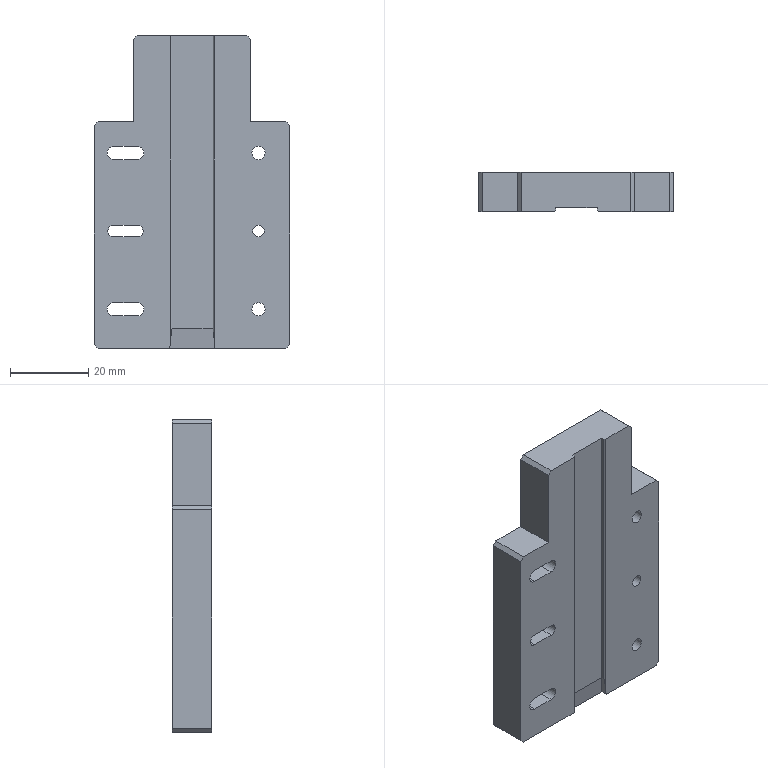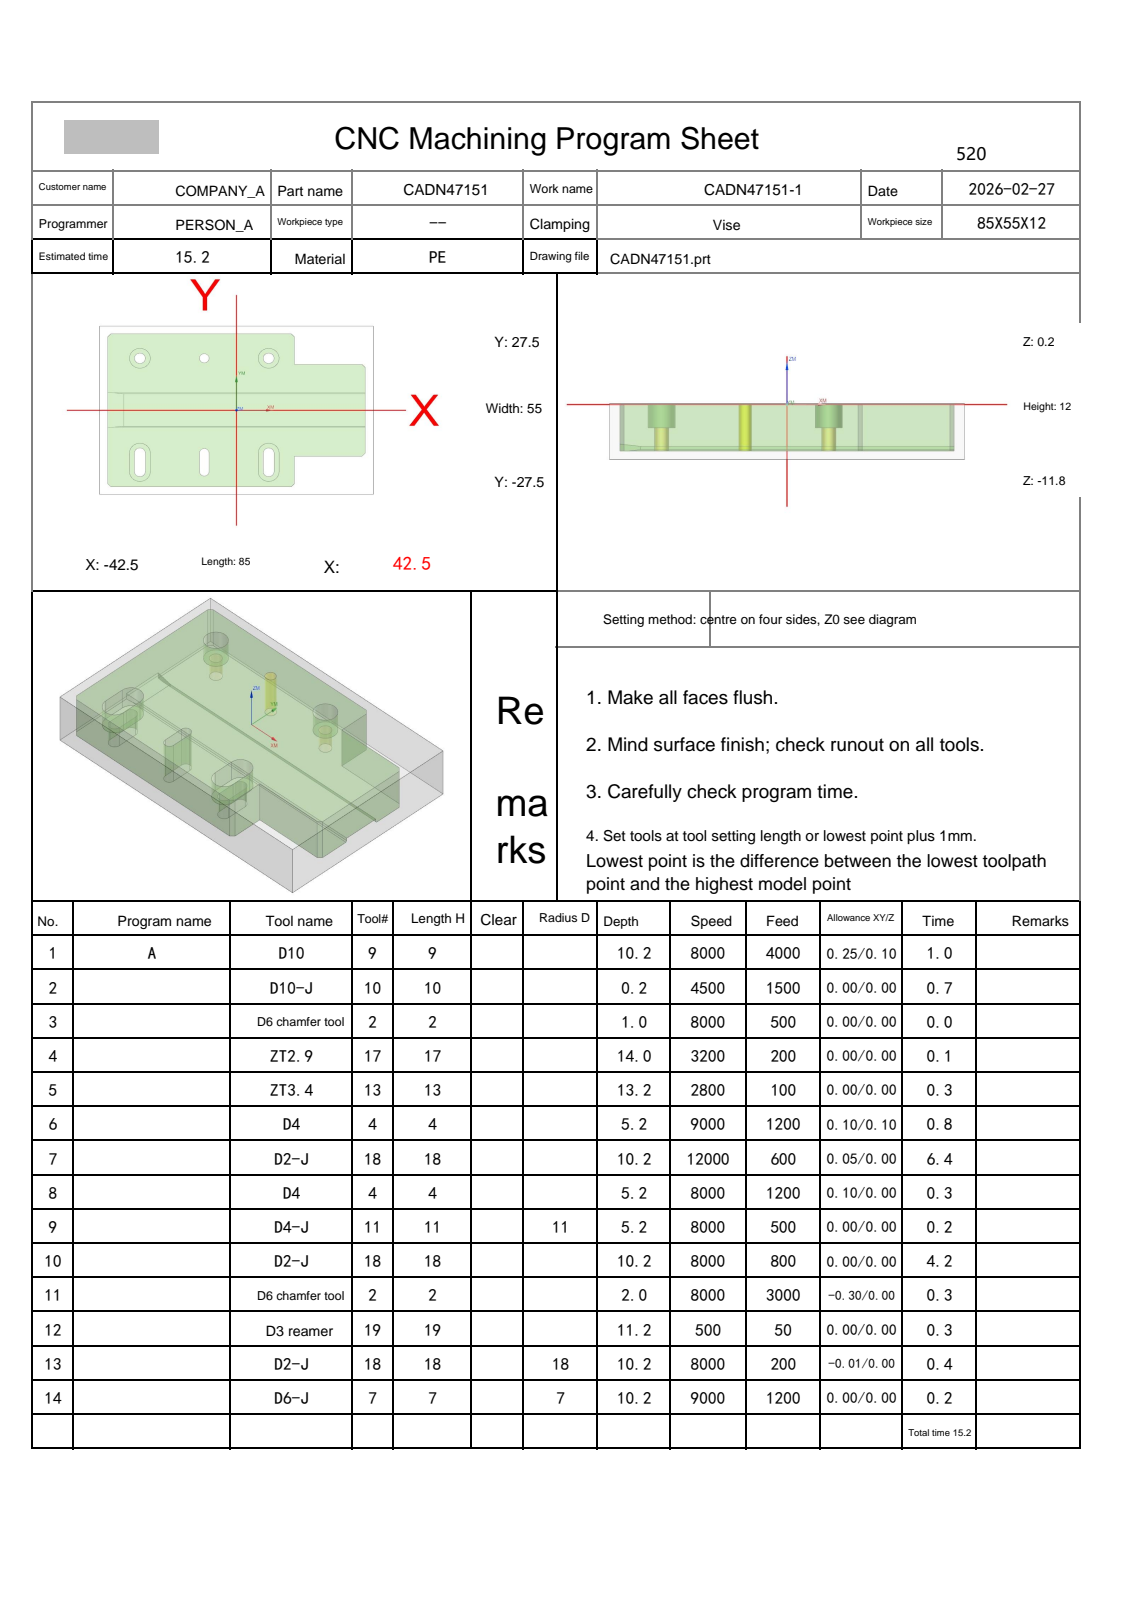NC program | NX | posted by the shop | part box 50 x 10 x 80 mm
Lines 1 to 1266 of 8100:
%
O0001
(Machine time: 17.84 MIN)
(===Total Tool:10===)
(T9=D10     D=10.  R=0.   D-  H09 Z=-10.  )
(T10=D10-J  D=10.  R=0.   D-  H10 Z=0.    )
(T2=D6 chamfer tool   D=6.   R=0.   D-  H02 Z=-1.8  )
(T17=ZT2.9  D=2.9  DR_a=120 D-  H17 Z=-13.84)
(T13=ZT3.4  D=3.4  DR_a=118 D-  H13 Z=-13.02)
(T4=D4      D=4.   R=0.   D-  H04 Z=-5.   )
(T18=D2-J   D=2.   R=0.   D-  H18 Z=-10.  )
(T11=D4-J   D=4.   R=0.   D11 H11 Z=-5.   )
(T19=D3 reamer   D=3.   DR_a=180 D-  H19 Z=-11.  )
(T7=D6-J    D=6.   R=0.   D7  H07 Z=-10.  )
G80 G90 G17 G49 G40
G91 G28 Z0
M01
N1 T09 M06
(D10  D=10. R=0. H=09 ce=0.25 di=0.10)
G00 G90 G54 X53.977 Y1.05 M03 S8000
G43 H09 Z50.
M08
Z-8.
G01 X53.878 Y1.032 Z-8.625 F4000.
X53.78 Y1.014 Z-8.872
X53.682 Y.996 Z-9.054
X53.583 Y.978 Z-9.2
X53.485 Y.96 Z-9.323
X53.387 Y.942 Z-9.428
X53.288 Y.924 Z-9.52
X53.19 Y.906 Z-9.6
X53.092 Y.888 Z-9.67
X52.993 Y.87 Z-9.732
X52.895 Y.852 Z-9.786
X52.796 Y.834 Z-9.833
X52.698 Y.816 Z-9.874
X52.6 Y.797 Z-9.908
X52.501 Y.779 Z-9.936
X52.403 Y.761 Z-9.96
X52.305 Y.743 Z-9.977
X52.206 Y.725 Z-9.99
X52.108 Y.707 Z-9.997
X52.01 Y.689 Z-10.
X49.894 Y.301
G03 X49.531 Y.025 I.097 J-.504
X49.097 Y-3.1 I11.047 J-3.125
G01 Y-3.168
G03 X48.997 Y-11.593 I354.863 J-8.424
X49. Y-13.006 I354.963 J0.0
G02 X49.015 Y-17.868 I-787.443 J-4.861
X48.97 Y-26.356 I-787.458 J0.0
X43.827 Y-33.039 I-7.224 J.238
X38.212 Y-33.904 I-5.806 J19.054
X29.259 Y-34.006 I-8.953 J392.015
X27.063 Y-34. I0.0 J392.117
G01 X-41.069 Y-33.984
X-41.096
G02 X-48.042 Y-28.819 I0.0 J7.254
X-48.914 Y-22.955 I19.689 J5.924
X-49.003 Y-13.772 I474.862 J9.182
X-49. Y-12.005 I474.951 J0.0
G01 X-48.984 Y26.069
Y26.096
G02 X-43.819 Y33.042 I7.254 J0.0
X-37.955 Y33.914 I5.924 J-19.689
X-28.772 Y34.003 I9.182 J-474.862
X-27.005 Y34. I0.0 J-474.951
G01 X41.069 Y33.984
X41.096
G02 X48.042 Y28.819 I0.0 J-7.254
X48.914 Y22.954 I-19.689 J-5.924
X49.021 Y10.694 I-707.018 J-12.261
X48.963 Y1.656 I-707.124 J0.0
G03 X48.498 Y-9.252 I127.706 J-10.908
X48.505 Y-10.615 I128.171 J0.0
G02 X48.521 Y-15.637 I-779.152 J-5.022
X48.465 Y-25.004 I-779.168 J0.0
X43.679 Y-31.936 I-7.896 J.334
X37.464 Y-33.313 I-6.835 J16.126
X28.561 Y-33.517 I-8.903 J194.629
X25.918 Y-33.499 I0.0 J194.833
G01 X-39.655 Y-33.482
G02 X-47.019 Y-28.497 I.029 J7.975
X-48.313 Y-22.465 I16.584 J6.714
X-48.52 Y-13.11 I211.138 J9.355
X-48.499 Y-10.118 I211.345 J0.0
G01 X-48.48 Y24.705
G02 X-43.679 Y31.935 I7.926 J-.053
X-37.465 Y33.313 I6.835 J-16.119
X-28.138 Y33.52 I9.327 J-210.133
X-25.168 Y33.499 I0.0 J-210.34
G01 X39.655 Y33.482
G02 X47.019 Y28.497 I-.029 J-7.975
X48.313 Y22.465 I-16.584 J-6.714
X48.52 Y13.11 I-211.138 J-9.355
X48.499 Y10.118 I-211.346 J0.0
X48.522 Y7.551 I-146.57 J-2.567
X48.169 Y-2.608 I-146.592 J0.0
G03 X48. Y-12.795 I306.009 J-10.187
G01 X48.001 Y-13.507
G02 X48.018 Y-17.014 I-360.035 J-3.507
X47.953 Y-23.855 I-360.052 J0.0
X42.658 Y-31.323 I-8.682 J.544
X36.005 Y-32.794 I-7.383 J17.622
X27.174 Y-33.012 I-8.83 J178.054
X24.909 Y-32.998 I0.0 J178.273
G01 X-38.241 Y-32.983
X-38.277
G02 X-46.322 Y-27.659 I0.0 J8.741
X-47.793 Y-21.005 I17.608 J7.383
X-48.014 Y-12.022 I182.708 J8.983
X-47.998 Y-9.609 I182.929 J0.0
G01 X-47.973 Y23.49
G02 X-42.659 Y31.322 I8.718 J-.196
X-36.005 Y32.793 I7.383 J-17.609
X-27.02 Y33.014 I8.985 J-182.767
X-24.609 Y32.998 I0.0 J-182.988
G01 X38.29 Y32.982
G02 X46.322 Y27.659 I-.01 J-8.737
X47.793 Y21.005 I-17.609 J-7.383
X48.014 Y12.022 I-182.711 J-8.983
X47.998 Y9.609 I-182.931 J0.0
X48.001 Y8.479 I-198.39 J-1.13
X47.65 Y-3.318 I-198.393 J0.0
G03 X47.478 Y-18.337 I654.031 J-15.019
X47.487 Y-21.806 I654.204 J0.0
G02 X47.49 Y-22.034 I-9.468 J-.228
X41.526 Y-30.832 I-9.471 J0.0
X34.809 Y-32.273 I-7.637 J19.219
X25.573 Y-32.513 I-9.236 J177.333
X23.214 Y-32.497 I0.0 J177.573
G01 X-37.036 Y-32.479
X-37.056
G02 X-45.825 Y-26.538 I0.0 J9.443
X-47.29 Y-19.574 I19.56 J7.75
X-47.517 Y-9.838 I208.749 J9.736
X-47.498 Y-7.028 I208.976 J0.0
G01 X-47.481 Y21.972
Y22.05
G02 X-41.538 Y30.826 I9.45 J0.0
X-34.574 Y32.29 I7.75 J-19.561
X-24.836 Y32.517 I9.738 J-208.817
X-22.028 Y32.498 I0.0 J-209.044
G01 X36.972 Y32.481
X37.05 Y32.482
G02 X45.826 Y26.538 I0.0 J-9.45
X47.29 Y19.574 I-19.562 J-7.75
X47.519 Y9.517 I-221.257 J-10.057
X47.178 Y-2.769 I-221.486 J0.0
G03 X46.979 Y-18.281 I604.501 J-15.512
X46.983 Y-20.656 I604.7 J0.0
G01 X46.985 Y-20.853
G02 X44.669 Y-27.375 I-10.342 J0.0
X38.251 Y-31.072 I-8.949 J8.117
X30.461 Y-31.919 I-7.882 J36.235
X20.214 Y-32. I-10.248 J651.166
X18.862 Y-31.998 I0.0 J651.247
G01 X-35.788 Y-31.978
X-35.917 Y-31.979
G02 X-43.02 Y-29.073 I0.0 J10.133
X-46.222 Y-22.617 I9.557 J8.763
X-46.941 Y-14.714 I43.079 J7.902
G01 Y-14.611
G02 X-47.002 Y-5.696 I655.87 J8.915
X-46.998 Y-3.611 I655.93 J0.0
G01 X-46.976 Y20.839
Y20.944
G02 X-43.67 Y28.392 I10.042 J0.0
X-37.126 Y31.321 I8.642 J-10.533
X-28.922 Y31.966 I8.204 J-51.84
X-28.361 Y31.963 I0.0 J-52.485
G01 X-18.611 Y31.998
X35.839 Y31.976
X35.943 Y31.977
G02 X43.156 Y28.924 I0.0 J-10.049
X46.242 Y22.511 I-9.842 J-8.686
X46.943 Y14.63 I-43.943 J-7.881
G01 Y14.503
G02 X46.985 Y9.735 I-270.462 J-4.768
X46.652 Y-3.693 I-270.504 J0.0
G03 X46.469 Y-19.857 I958.738 J-18.923
G01 Y-19.878
G02 X43.937 Y-26.81 I-10.755 J0.0
X37.405 Y-30.524 I-9.213 J8.603
X29.071 Y-31.421 I-8.335 J38.26
X18.93 Y-31.5 I-10.14 J655.907
X17.471 Y-31.498 I0.0 J655.986
G01 X-34.529 Y-31.479
X-34.6
G02 X-40.239 Y-30.093 I0.0 J12.161
X-43.188 Y-28.258 I1.605 J5.867
X-45.308 Y-24.357 I4.303 J4.865
X-46.419 Y-14.388 I46.553 J10.234
X-46.5 Y-4.081 I657.762 J10.307
X-46.498 Y-2.488 I657.843 J0.0
G01 X-46.471 Y19.761
G02 X-45.092 Y25.246 I11.999 J-.101
X-43.711 Y27.713 I5.537 J-1.479
G01 X-42.085 Y29.248
G02 X-39.342 Y30.31 I3.668 J-5.402
X-29.122 Y31.426 I10.327 J-47.201
X-19.247 Y31.5 I9.875 J-657.174
X-17.523 Y31.498 I0.0 J-657.249
G01 X34.527 Y31.479
X34.716 Y31.481
G02 X40.917 Y29.635 I0.0 J-11.339
X45.313 Y23.168 I-6.959 J-9.458
X46.376 Y15.411 I-30.851 J-8.178
X46.467 Y8.759 I-241.853 J-6.651
X46.172 Y-3.194 I-241.945 J0.0
G03 X45.97 Y-18.711 I841.279 J-18.691
G01 Y-18.771
G02 X43.979 Y-25.318 I-11.761 J0.0
X37.436 Y-29.748 I-9.705 J7.286
X29.635 Y-30.858 I-8.374 J30.89
X18.907 Y-31.009 I-10.728 J382.487
X15.987 Y-30.998 I0.0 J382.637
G01 X-33.363 Y-30.979
G02 X-38.013 Y-30.25 I.115 J15.922
X-38.514 Y-30.264 I-.502 J8.744
X-40.242 Y-30.092 I0.0 J8.758
G03 X-38.262 Y-30.272 I1.98 J10.806
X-37.667 Y-30.256 I0.0 J10.986
X-29.407 Y-30.607 I8.261 J97.074
X-27.82 Y-30.594 I0.0 J97.425
G01 X23.634 Y-30.58
G03 X24.704 Y-30.588 I1.071 J78.351
X33.664 Y-30.074 I0.0 J78.359
X40.558 Y-27.693 I-1.817 J16.438
X45.22 Y-20.113 I-6.075 J8.961
X45.6 Y-14.16 I-46.482 J5.954
X45.597 Y-13.63 I-46.861 J0.0
G02 X46.044 Y5.056 I741.844 J-8.393
G03 X46.1 Y8.875 I-130.374 J3.819
X45.784 Y17.948 I-130.43 J0.0
X44.034 Y24.942 I-19.775 J-1.23
X35.837 Y30.742 I-9.415 J-4.614
X29.577 Y31.103 I-6.261 J-54.029
X28.402 Y31.09 I0.0 J-54.39
G01 X-26.248 Y31.07
G03 X-26.865 Y31.073 I-.617 J-71.011
X-36.22 Y30.454 I0.0 J-71.014
G02 X-38.426 Y30.226 I-2.205 J10.558
X-39.125 Y30.248 I0.0 J10.786
G01 X-40.348 Y30.076
G02 X-38.165 Y30.269 I2.182 J-12.221
X-37.444 Y30.248 I0.0 J-12.415
G03 X-29.913 Y30.477 I-.343 J135.653
G02 X-17.911 Y30.602 I12.002 J-573.446
X-15.514 Y30.597 I0.0 J-573.572
G01 X29.736 Y30.574
G02 X30.362 Y30.58 I.626 J-30.941
X36.151 Y30.034 I0.0 J-30.947
X43.939 Y23.116 I-2.436 J-10.586
X45.373 Y15.731 I-23.454 J-8.387
X45.569 Y7.889 I-157.392 J-7.841
X45.42 Y1.036 I-157.587 J0.0
G03 X45.226 Y-10.074 I318.081 J-11.11
X45.25 Y-14.002 I318.275 J0.0
G02 X44.671 Y-19.744 I-58.173 J2.965
X37.39 Y-28.391 I-11.087 J1.946
X29.712 Y-29.87 I-8.649 J24.235
X20.007 Y-30.105 I-9.705 J200.151
X18.166 Y-30.097 I0.0 J200.386
G01 X17.2 Y-30.246
X-37.85 Y-30.25
G03 X-38.35 Y-30.75 I0.0 J-.5
X-38.119 Y-31.171 I.5 J0.0
G01 X-37.372 Y-31.648
X-35.701 Y-32.714 Z-9.9
X-35.361 Y-32.931
X-35.298 Y-32.965
X-35.232 Y-32.99
X-35.162 Y-33.005
X-35.091 Y-33.01
X15.407 Y-32.856
X15.491 Y-32.849
X15.573 Y-32.827
X15.649 Y-32.793
X15.719 Y-32.745
X17.018 Y-31.248 Z-10.
X17.913 Y-30.215
G02 X19.428 Y-29.888 I1.63 J-3.884
X27.197 Y-29.583 I9.717 J-148.644
G03 X35.168 Y-28.581 I-.47 J35.935
X41.784 Y-24.496 I-2.893 J12.085
X44.376 Y-17.974 I-10.749 J8.048
G01 X44.577 Y-16.551
X45.071 Y-15.359
X45.25 Y-14.002
X45.071 Y-15.359
G03 X43.532 Y-19.678 I31.519 J-13.668
G02 X35.394 Y-27.742 I-11.687 J3.654
X27.37 Y-29.028 I-8.8 J29.24
G03 X20.119 Y-29.381 I4.644 J-170.313
X19.579 Y-29.573 I.054 J-1.006
G01 X18.433 Y-30.056
X20.126 Y-29.304
G02 X24.435 Y-28.786 I4.653 J-20.498
G03 X32.477 Y-28.004 I-1.448 J56.619
X39.37 Y-24.881 I-2.445 J14.566
X43.163 Y-19.067 I-9.393 J10.273
G01 X43.711 Y-17.713
X44.547 Y-16.625
G03 X42.144 Y-20.306 I14.839 J-12.309
G02 X33.291 Y-27.106 I-12.178 J6.691
X25.48 Y-28.203 I-9.377 J38.403
G03 X20.68 Y-28.794 I.698 J-25.485
G01 X19.759 Y-29.454
X20.718 Y-28.749
G02 X24.207 Y-27.973 I4.129 J-10.327
G03 X31.46 Y-27.058 I-5.462 J72.542
X38.937 Y-23.434 I-2.695 J15.084
X42.344 Y-19.023 I-15.379 J15.399
X43.711 Y-17.713 I-23.663 J26.076
G02 X41.901 Y-19.405 I-20.641 J20.268
X38.549 Y-22.928 I-29.336 J24.562
X30.687 Y-26.561 I-10.91 J13.285
X23.882 Y-27.533 I-18.611 J106.014
G03 X21.213 Y-28.23 I.799 J-8.517
G01 X20.578 Y-28.832
G02 X23.057 Y-27.445 I3.203 J-2.816
X28.876 Y-26.461 I17.86 J-87.913
G03 X36.584 Y-23.687 I-2.784 J19.829
X40.888 Y-19.884 I-14.851 J21.148
G01 X41.625 Y-19.547
X42.339 Y-18.999
G02 X40.781 Y-19.912 I-3.047 J3.411
G03 X37.595 Y-22.289 I39.735 J-56.585
G02 X28.754 Y-25.882 I-12.372 J17.771
G03 X23.192 Y-26.983 I11.673 J-73.551
X21.843 Y-27.549 I.98 J-4.223
G01 X21.24 Y-28.204
G02 X22.181 Y-27.271 I4.795 J-3.9
X25.782 Y-26.085 I5.47 J-10.547
G03 X32.485 Y-24.402 I-8.054 J46.254
X38.795 Y-20.816 I-8.901 J23.008
G02 X39.868 Y-20.136 I4.281 J-5.568
G03 X40.959 Y-19.822 I-.116 J2.464
G02 X39.626 Y-20.19 I-1.762 J3.782
G03 X36.381 Y-21.916 I9.596 J-21.955
G02 X27.58 Y-25.153 I-14.713 J26.42
G03 X22.998 Y-26.476 I4.424 J-23.917
X22.425 Y-26.825 I1.547 J-3.186
G01 X21.861 Y-27.527
G02 X24.152 Y-25.798 I3.489 J-2.241
X29.571 Y-24.234 I23.148 J-70.025
G03 X37.374 Y-20.864 I-10.099 J34.105
G02 X38.733 Y-20.25 I5.626 J-10.641
G01 X39.841 Y-20.139
G03 X38.186 Y-20.331 I5.071 J-51.09
X34.274 Y-21.93 I9.978 J-29.979
G02 X26.523 Y-24.536 I-22.319 J53.569
G03 X22.908 Y-26.066 I2.815 J-11.686
X22.43 Y-26.814 I1.245 J-1.321
G02 X23.885 Y-25.296 I2.54 J-.977
X27.912 Y-23.757 I10.204 J-20.655
G03 X36.144 Y-20.679 I-22.277 J72.129
G01 X37.427 Y-20.25
X38.677
G03 X38.02 Y-20.225 I-.657 J-8.735
X34.671 Y-20.891 I0.0 J-8.759
G02 X26.073 Y-23.868 I-231.278 J654.106
G03 X23.063 Y-25.515 I2.739 J-8.58
G01 X22.709 Y-26.252
G02 X23.224 Y-25.284 I3.786 J-1.393
X26.174 Y-23.52 I5.738 J-6.248
X35.259 Y-20.327 I64.878 J-170.115
G01 X35.587 Y-20.25
X37.237
G03 X36.388 Y-20.226 I-.848 J-14.798
X34.245 Y-20.382 I0.0 J-14.822
X25.181 Y-23.51 I11.561 J-48.193
X23.15 Y-25.05 I2.185 J-4.993
G01 X22.979 Y-25.655
G02 X24.108 Y-23.948 I2.467 J-.406
X28.539 Y-21.763 I9.789 J-14.261
X33.345 Y-20.25 I16.134 J-42.871
G01 X35.245
G03 X34.262 Y-20.227 I-.983 J-21.383
X32.06 Y-20.341 I0.0 J-21.405
X24.604 Y-23.169 I3.922 J-21.582
X23.221 Y-24.55 I1.951 J-3.336
G01 X23.124 Y-25.111
G02 X24.099 Y-23.342 I2.393 J-.165
X28.677 Y-20.921 I8.832 J-11.163
X30.977 Y-20.25 I10.629 J-32.146
G01 X32.927
G03 X31.937 Y-20.229 I-.989 J-23.118
X29.846 Y-20.324 I0.0 J-23.139
X24. Y-23.025 I2.001 J-12.006
X23.247 Y-24.086 I1.565 J-1.909
G01 X23.211 Y-24.605
X23.21 Y-24.544
G02 X24.054 Y-22.765 I2.295 J0.0
X28.894 Y-20.25 I7.243 J-8.022
G01 X30.544
G03 X29.724 Y-20.226 I-.82 J-13.844
X27.88 Y-20.349 I0.0 J-13.869
X23.602 Y-22.885 I1.565 J-7.517
X23.231 Y-23.83 I1.019 J-.946
X23.248 Y-24.05 I1.39 J0.0
G02 X23.238 Y-23.849 I2.073 J.201
X23.892 Y-22.334 I2.083 J0.0
X27.365 Y-20.25 I5.343 J-4.968
G01 X28.615
G03 X28.002 Y-20.226 I-.613 J-7.851
X26.465 Y-20.377 I0.0 J-7.875
X23.277 Y-22.872 I1.292 J-4.936
G01 X23.25 Y-23.554
G02 X23.237 Y-23.318 I2.218 J.236
X24.008 Y-21.632 I2.231 J0.0
X26.271 Y-20.25 I3.751 J-3.599
G01 X27.171
G03 X26.722 Y-20.225 I-.448 J-4.025
X25.027 Y-20.597 I0.0 J-4.05
X23.256 Y-22.421 I1.517 J-3.245
G01 X23.25 Y-22.971
G02 X23.239 Y-22.76 I2.093 J.211
X24.038 Y-21.11 I2.104 J0.0
X25.5 Y-20.25 I2.516 J-2.605
G01 X26.2
G03 X25.841 Y-20.227 I-.36 J-2.784
X23.257 Y-21.936 I0.0 J-2.808
G01 X23.25 Y-22.436
X23.241 Y-22.252
G02 X24.101 Y-20.675 I1.876 J0.0
X25.212 Y-20.235 I1.111 J-1.181
X25.432 Y-20.25 I0.0 J-1.622
G03 X25.135 Y-20.228 I-.296 J-1.963
X23.25 Y-21.592 I0.0 J-1.985
G01 Y-21.942
X23.245 Y-21.812
G02 X24.186 Y-20.37 I1.576 J0.0
X24.722 Y-20.24 I.536 J-1.043
G01 X24.874 Y-20.25
G03 X24.655 Y-20.233 I-.22 J-1.447
X23.25 Y-21.285 I0.0 J-1.464
G01 Y-21.585
X23.241 Y-21.439
G02 X24.431 Y-20.249 I1.19 J0.0
G01 X24.482 Y-20.25
X24.322 Y-20.239
G03 X23.25 Y-21.052 I0.0 J-1.114
G01 Y-21.252
X23.245 Y-21.161
G02 X24.157 Y-20.249 I.911 J0.0
G01 X24.193 Y-20.25
X24.049 Y-20.237
G03 X23.249 Y-21.037 I0.0 J-.8
G01 X23.25 Y-21.072
X23.243 Y-20.972
G02 X23.966 Y-20.249 I.723 J0.0
G01 X24.003 Y-20.25
X23.887 Y-20.239
G03 X23.249 Y-20.877 I0.0 J-.637
G01 X23.25 Y-20.903
G03 X23.396 Y-21.257 I.52 J.008
G01 X24.326 Y-22.186
X25.727 Y-23.588 Z-9.9
X26.05 Y-23.911
X26.11 Y-23.962
X26.177 Y-24.003
X26.249 Y-24.033
X26.326 Y-24.051
X26.404 Y-24.057
X31.64
X32.487 Y-24.05
X33.335 Y-24.028
X34.181 Y-23.992
X35.028 Y-23.941
X35.873 Y-23.876
X36.716 Y-23.796
X37.559 Y-23.702
X38.399 Y-23.593
X39.238 Y-23.47
X40.074 Y-23.333
X40.908 Y-23.181
X44.284 Y-22.537
X44.472 Y-22.494
X44.657 Y-22.438
X44.837 Y-22.367
X45.011 Y-22.285
X45.179 Y-22.189
X45.339 Y-22.081
X45.491 Y-21.963
X45.634 Y-21.833
X45.767 Y-21.693
X45.89 Y-21.544
X46.001 Y-21.386
X46.1 Y-21.221
X46.293 Y-20.857
X46.474 Y-20.487
X46.642 Y-20.112
X46.798 Y-19.731
X46.94 Y-19.345
X47.07 Y-18.954
X47.637 Y-17.142
X47.785 Y-16.645
X47.919 Y-16.145
X48.039 Y-15.641
X48.146 Y-15.134
X48.239 Y-14.624
X48.317 Y-14.112
X48.382 Y-13.598
X48.432 Y-13.082
X48.468 Y-12.565
X48.49 Y-12.047
X48.498 Y-11.529
X48.491 Y-11.011
X48.404 Y-7.704
X48.395 Y-7.621
X48.372 Y-7.541
X48.336 Y-7.466
X48.288 Y-7.398
X48.23 Y-7.338
X47.741 Y-6.918
X46.237 Y-5.627 Z-10.
X45.364 Y-4.868
X45.25 Y-4.551
Y14.
G03 X44.295 Y20.269 I-64.76 J-6.658
X40.934 Y26.647 I-12.695 J-2.615
X34.403 Y29.733 I-8.117 J-8.723
X27.677 Y30.188 I-6.727 J-49.584
X26.874 Y30.181 I0.0 J-50.039
G01 X17.515 Y30.198
X17.203 Y30.246
X-35.297 Y30.248
G02 X-35.796 Y30.748 I0.0 J.5
X-35.565 Y31.17 I.5 J0.0
G01 X-34.815 Y31.649
X-33.143 Y32.714 Z-9.9
X-32.806 Y32.929
X-32.744 Y32.963
X-32.677 Y32.988
X-32.608 Y33.003
X-32.537 Y33.008
X14.756 Y32.957
X14.841 Y32.95
X14.924 Y32.928
X15.002 Y32.892
X15.073 Y32.843
X15.134 Y32.783
X15.172 Y32.74
X16.464 Y31.237 Z-10.
X17.262 Y30.316
G03 X18.433 Y30.056 I1.273 J2.967
X23.469 Y29.709 I5.036 J36.439
X24.116 Y29.715 I0.0 J36.785
G02 X24.988 Y29.719 I.872 J-90.757
X32.596 Y29.4 I0.0 J-90.761
X39.039 Y27.135 I-1.058 J-13.307
X43.449 Y20.606 I-7.497 J-9.817
X44.301 Y16.958 I-44.736 J-12.379
G01 X44.547 Y16.625
X45.071 Y15.359
G03 X44.199 Y17.14 I-6.362 J-2.011
G01 X42.792 Y21.117
G03 X33.867 Y28.601 I-11.099 J-4.172
X26.539 Y29.273 I-7.328 J-39.674
X26.209 Y29.271 I0.0 J-40.345
G02 X25.707 Y29.269 I-.501 J63.706
X19.594 Y29.563 I0.0 J63.708
G01 X18.433 Y30.056
G03 X22.768 Y28.962 I4.592 J9.063
G02 X30.418 Y28.544 I-14.028 J-326.874
X37.053 Y26.664 I-1.01 J-16.22
X42.159 Y20.737 I-6.518 J-10.777
G01 X43.287 Y18.137
G02 X44.322 Y16.918 I-5.747 J-5.925
G03 X43.115 Y18.344 I-11.421 J-8.444
G02 X41.219 Y21.633 I110.135 J65.669
G03 X32.496 Y27.674 I-11.08 J-6.68
X25.122 Y28.425 I-8.376 J-45.721
G02 X20.411 Y29.009 I.253 J21.335
G01 X19.592 Y29.564
G03 X21.039 Y28.688 I4.28 J5.434
X25.68 Y27.947 I5.396 J18.874
G02 X32.403 Y27.069 I-1.95 J-41.141
X40.702 Y21.123 I-3.122 J-13.12
G01 X41.896 Y19.339
G02 X43.279 Y18.145 I-4.841 J-7.01
G03 X41.69 Y19.516 I-8.895 J-8.71
G01 X39.097 Y22.491
G03 X30.773 Y26.866 I-10.796 J-10.433
X24.142 Y27.707 I-15.158 J-92.966
G02 X20.952 Y28.486 I.818 J10.275
G01 X20.336 Y29.041
G03 X23.141 Y27.557 I3.608 J3.425
X28.798 Y26.664 I16.159 J84.002
G02 X36.177 Y24.007 I-2.21 J-17.715
X40.124 Y20.435 I-14.101 J-19.547
G01 X40.648 Y19.951
G02 X41.823 Y19.394 I-1.267 J-4.192
G03 X40.556 Y19.991 I-2.702 J-4.097
G02 X37.971 Y22.063 I13.884 J19.968
G03 X28.869 Y26.158 I-11.992 J-14.495
G02 X23.188 Y27.207 I12.554 J83.849
X21.602 Y27.828 I1.926 J7.253
G01 X21.014 Y28.427
G03 X23.725 Y26.77 I3.808 J3.185
X29.313 Y25.529 I26.399 J105.711
G02 X37.554 Y21.601 I-4.26 J-19.544
G03 X39.599 Y20.171 I7.951 J9.195
G01 X39.616
G02 X40.636 Y19.956 I0.0 J-2.527
G03 X39.5 Y20.188 I-1.266 J-3.311
G02 X37.712 Y21.139 I3.535 J8.803
G03 X27.371 Y25.495 I-15.265 J-21.785
G02 X22.832 Y26.783 I4.215 J23.498
X21.665 Y27.762 I.904 J2.262
G03 X24.155 Y25.987 I3.788 J2.679
X29.442 Y24.455 I28.065 J86.957
G02 X36.833 Y21.056 I-8.878 J-29.045
G03 X38.461 Y20.25 I4.688 J7.415
G01 X38.485
G02 X39.596 Y20.171 I0.0 J-7.921
G03 X38.193 Y20.285 I-3.358 J-32.74
G02 X34.835 Y21.781 I6.016 J18.018
G03 X26.773 Y24.76 I-18.297 J-37.119
G02 X22.817 Y26.34 I3.388 J14.223
X22.425 Y26.825 I.539 J.837
G01 X22.174 Y27.137
G02 X22.678 Y26.388 I-6.098 J-4.656
G03 X25.416 Y24.814 I4.925 J5.395
G02 X31.811 Y22.546 I-53.266 J-160.31
G03 X36.773 Y20.345 I108.837 J238.792
G01 X37.105 Y20.25
X38.455
G02 X37.843 Y20.225 I-.611 J7.581
X36.216 Y20.401 I0.0 J7.606
X31.415 Y22.258 I23.205 J67.151
X25.147 Y24.546 I95.993 J272.682
X22.843 Y25.98 I2.279 J6.229
G01 X22.555 Y26.563
G03 X24.398 Y24.607 I3.45 J1.405
X28.223 Y22.93 I12.975 J24.385
X35.013 Y20.335 I132.535 J336.577
G01 X35.335 Y20.25
X37.035
G02 X36.267 Y20.227 I-.768 J13.189
X34.543 Y20.341 I0.0 J13.211
X29.005 Y22.214 I12.523 J46.139
X24.226 Y24.374 I8.25 J24.619
X23.039 Y25.456 I1.735 J3.094
G01 X22.886 Y25.894
G03 X24.271 Y24.073 I2.996 J.842
X29.095 Y21.697 I12.34 J18.973
X33.253 Y20.25 I16.918 J41.907
G01 X35.203
G02 X34.314 Y20.225 I-.889 J16.008
X32.311 Y20.351 I0.0 J16.032
X24.631 Y23.475 I5.68 J24.962
X23.162 Y24.931 I2.17 J3.662
G01 X23.052 Y25.409
G03 X24.244 Y23.48 I2.895 J.456
X29.211 Y20.841 I10.444 J13.665
X31.074 Y20.25 I21.518 J64.567
G01 X33.124
G02 X32.214 Y20.229 I-.911 J19.808
X30.292 Y20.322 I0.0 J19.829
X24.051 Y23.319 I2.708 J13.637
X23.227 Y24.433 I2.041 J2.373
G01 X23.166 Y24.909
G03 X24.193 Y22.905 I2.781 J.161
X29.124 Y20.25 I8.059 J9.06
G01 X30.974
G02 X30.165 Y20.231 I-.809 J17.451
X28.519 Y20.309 I0.0 J17.47
X23.686 Y23.14 I1.81 J8.633
X23.225 Y24.295 I1.218 J1.155
G01 X23.229 Y24.406
X23.228 Y24.344
G03 X24.118 Y22.363 I2.65 J0.0
X27.594 Y20.25 I5.915 J5.814
G01 X28.994
G02 X28.377 Y20.228 I-.617 J8.744
X27.007 Y20.336 I0.0 J8.765
X23.327 Y23.174 I1.433 J5.664
X23.235 Y23.704 I1.493 J.53
X23.25 Y23.919 I1.584 J0.0
G01 X23.242 Y23.721
G03 X24.104 Y21.782 I2.615 J0.0
X26.478 Y20.25 I4.186 J3.882
G01 X27.578
G02 X27.088 Y20.227 I-.49 J5.192
X25.908 Y20.362 I0.0 J5.215
X23.254 Y22.837 I1.289 J4.043
G01 X23.25 Y23.371
G03 X23.241 Y23.161 I2.577 J-.209
X24.195 Y21.156 I2.585 J0.0
X25.664 Y20.25 I2.662 J2.672
G01 X26.464
G02 X26.104 Y20.228 I-.36 J2.94
X23.608 Y21.594 I0.0 J2.962
X23.238 Y22.596 I1.169 J1.002
G01 X23.25 Y22.789
X23.242 Y22.602
G03 X24.279 Y20.663 I2.331 J0.0
X25.393 Y20.229 I1.114 J1.212
X25.656 Y20.25 I0.0 J1.646
G02 X25.389 Y20.234 I-.266 J2.184
X23.45 Y21.396 I0.0 J2.2
X23.235 Y22.09 I1.017 J.694
G01 X23.25 Y22.279
X23.241 Y22.096
G03 X24.62 Y20.25 I1.925 J0.0
G01 X25.02
X24.851 Y20.241
G02 X23.25 Y21.5 I0.0 J1.648
G01 Y21.85
X23.238 Y21.662
G03 X24.295 Y20.25 I1.472 J0.0
G01 X24.595
X24.436 Y20.239
G02 X23.249 Y21.426 I0.0 J1.187
G01 X23.25 Y21.467
X23.232 Y21.275
G03 X24.258 Y20.249 I1.026 J0.0
G01 X24.307 Y20.25
X24.168 Y20.239
G02 X23.249 Y21.158 I0.0 J.919
G01 X23.25 Y21.19
X23.238 Y21.054
G03 X24.043 Y20.249 I.805 J0.0
G01 X24.085 Y20.25
X23.99 Y20.244
G02 X23.287 Y20.712 I0.0 J.762
X23.25 Y20.908 I.514 J.196
X23.8 Y21.458 I.55 J0.0
X24.233 Y21.248 I0.0 J-.55
X24.428 Y20.798 I-.42 J-.45
X24.38 Y20.559 I-.615 J0.0
X23.885 Y20.25 I-.497 J.244
X23.4 Y20.482 I.053 J.736
X23.281 Y20.808 I.388 J.326
X23.788 Y21.315 I.507 J0.0
X24.164 Y21.148 I0.0 J-.507
X24.351 Y20.756 I-.316 J-.391
X23.848 Y20.253 I-.503 J0.0
G01 X23.701 Y20.275
G02 X23.24 Y20.892 I.182 J.617
G01 X23.25 Y21.003
G02 X23.425 Y21.384 I.513 J-.006
G01 X24.209 Y22.053
X25.717 Y23.34 Z-9.9
X26.229 Y23.777
X26.289 Y23.839
X26.338 Y23.91
X26.374 Y23.988
X26.396 Y24.071
X26.404 Y24.157
Y27.927
X26.396 Y28.109
X26.374 Y28.289
X26.337 Y28.466
X26.286 Y28.64
X26.221 Y28.81
X26.142 Y28.973
X26.05 Y29.129
X25.945 Y29.277
X25.829 Y29.417
X25.701 Y29.546
X25.564 Y29.664
X25.417 Y29.771
X24.342 Y30.488
X23.882 Y30.786
X23.415 Y31.073
X22.941 Y31.348
X22.46 Y31.612
X21.972 Y31.863
X21.479 Y32.102
X20.98 Y32.329
X20.475 Y32.543
X19.965 Y32.745
X19.386 Y32.966
X18.944 Y33.127
X18.497 Y33.276
X18.046 Y33.413
X17.591 Y33.537
X17.133 Y33.648
X16.672 Y33.746
X16.209 Y33.832
X15.743 Y33.904
X15.276 Y33.963
X14.807 Y34.01
X14.337 Y34.043
X13.866 Y34.062
X13.395 Y34.069
X-34.664
X-35.219 Y34.062
X-35.774 Y34.041
X-36.328 Y34.006
X-36.881 Y33.957
X-37.433 Y33.894
X-37.983 Y33.817
X-38.531 Y33.726
X-39.076 Y33.621
X-39.619 Y33.503
X-40.158 Y33.37
X-40.694 Y33.225
X-41.226 Y33.065
X-42.953 Y32.525
X-43.189 Y32.444
X-43.42 Y32.351
X-43.646 Y32.245
X-43.865 Y32.128
X-44.079 Y31.999
X-44.285 Y31.859
X-44.483 Y31.708
X-44.673 Y31.547
X-44.854 Y31.376
X-45.025 Y31.195
X-45.187 Y31.006
X-45.339 Y30.808
X-46.247 Y29.554
X-46.288 Y29.487
X-46.317 Y29.414
X-46.336 Y29.337
X-46.342 Y29.259
X-46.335 Y29.18
X-46.316 Y29.104
X-46.173 Y28.672
X-45.551 Y26.79 Z-10.
X-45.095 Y25.395
G02 X-45.512 Y23.35 I-13.766 J1.742
G03 X-46.084 Y17.031 I34.63 J-6.319
X-46.077 Y16.335 I35.202 J0.0
G01 X-46.076 Y-10.664
G03 X-46.081 Y-11.534 I75.586 J-.87
X-45.474 Y-21.088 I75.591 J0.0
G02 X-45.228 Y-23.341 I-10.155 J-2.252
X-45.25 Y-24.022 I-10.402 J0.0
G01 X-45.081 Y-25.334
G02 X-45.272 Y-23.177 I12.041 J2.157
X-45.25 Y-22.436 I12.233 J0.0
G03 X-45.479 Y-14.862 I-138.339 J-.383
G02 X-45.602 Y-2.798 I588.155 J12.064
X-45.597 Y-.363 I588.279 J0.0
X-45.62 Y5.646 I796.949 J6.009
X-45.524 Y18.036 I796.971 J0.0
X-45.25 Y21.372 I49.095 J-2.349
G01 Y24.025
X-45.103 Y25.165
X-45.25 Y24.025
Y-20.328
G02 X-45.756 Y-20.833 I-.506 J.001
G01 X-45.8 Y-20.831
X-47.728 Y-20.656
X-47.827 Y-20.647 Z-9.997
X-47.927 Y-20.638 Z-9.99
X-48.027 Y-20.629 Z-9.977
X-48.126 Y-20.62 Z-9.96
X-48.226 Y-20.611 Z-9.936
X-48.325 Y-20.602 Z-9.908
X-48.425 Y-20.593 Z-9.874
X-48.525 Y-20.584 Z-9.833
X-48.624 Y-20.575 Z-9.786
X-48.724 Y-20.566 Z-9.732
X-48.823 Y-20.557 Z-9.67
X-48.923 Y-20.548 Z-9.6
X-49.023 Y-20.539 Z-9.52
X-49.122 Y-20.53 Z-9.428
X-49.222 Y-20.521 Z-9.323
X-49.321 Y-20.512 Z-9.2
X-49.421 Y-20.503 Z-9.054
X-49.521 Y-20.494 Z-8.872
X-49.62 Y-20.485 Z-8.625
X-49.72 Y-20.476 Z-8.
G00 Z50.
G91 G28 Z0.0
M05
M09
G91 G28 Z0.0
M01
N2 T10 M06
(D10-J  D=10. R=0. H=10 ce=0.00 di=0.00)
G00 G90 G54 X-50. Y15.625 M03 S4500
G43 H10 Z50.
M08
Z2.
G01 Z0.0 F1500.
X-45. Y20.625
X-35.625 Y30.
X-26.25
X-45. Y11.25
Y1.875
X-16.875 Y30.
X-7.5
X-45. Y-7.5
Y-16.875
X1.875 Y30.
X11.25
X-45. Y-26.25
Y-30.
X-39.375
X20.625 Y30.
X30.
X-30. Y-30.
X-20.625
X39.375 Y30.
X45.
Y26.25
X-11.25 Y-30.
X-1.875
X45. Y16.875
Y7.5
X7.5 Y-30.
X16.875
X45. Y-1.875
Y-11.25
X26.25 Y-30.
X35.625
X45. Y-20.625
X50. Y-15.625
Z2.
G00 Z50.
G91 G28 Z0.0
M05
M09
G91 G28 Z0.0
M01
N3 T02 M06
(D6 chamfer tool  D=6. R=0. H=02 ce=0.00 di=0.00)
G00 G90 G54 X10. Y17. M03 S8000
G43 H02 Z50.
M08
G98 G81 X10. Y17. Z-.8 R1. F500.
X-10.
X-30.
G80
G00 Z50.
G91 G28 Z0.0
M05
M09
G91 G28 Z0.0
M01
N4 T17 M06
(ZT2.9 D=2.9 DR_a=120 H=17)
G00 G90 G54 X-10. Y17. M03 S3200
G43 H17 Z50.
M08
G98 G83 X-10. Y17. Z-13.837 R1. F200. Q2.
G80
G00 Z50.
G91 G28 Z0.0
M05
M09
G91 G28 Z0.0
M01
N5 T13 M06
(ZT3.4 D=3.4 DR_a=118 H=13)
G00 G90 G54 X10. Y17. M03 S2800
G43 H13 Z50.
M08
G98 G83 X10. Y17. Z-13.021 R1. F100. Q2.
X-30.
G80
G00 Z50.
G91 G28 Z0.0
M05
M09
G91 G28 Z0.0
M01
N6 T04 M06
(D4  D=4. R=0. H=04 ce=0.10 di=0.10)
G00 G90 G54 X11.15 Y-17. M03 S9000
G43 H04 Z50.
M08
Z.5
G01 Y-14. Z.461 F1200.
G03 X10. Y-12.85 Z.438 I-1.15 J0.0
X8.85 Y-14. Z.414 I0.0 J-1.15
G01 Y-20. Z.336
G03 X10. Y-21.15 Z.313 I1.15 J0.0
X11.15 Y-20. Z.289 I0.0 J1.15
G01 Y-14. Z.211
G03 X10. Y-12.85 Z.188 I-1.15 J0.0
X8.85 Y-14. Z.164 I0.0 J-1.15
G01 Y-20. Z.086
G03 X10. Y-21.15 Z.063 I1.15 J0.0
X11.15 Y-20. Z.039 I0.0 J1.15
G01 Y-14. Z-.039
G03 X10. Y-12.85 Z-.063 I-1.15 J0.0
X8.85 Y-14. Z-.086 I0.0 J-1.15
G01 Y-20. Z-.164
G03 X10. Y-21.15 Z-.188 I1.15 J0.0
X11.15 Y-20. Z-.211 I0.0 J1.15
G01 Y-14. Z-.289
G03 X10. Y-12.85 Z-.313 I-1.15 J0.0
X8.85 Y-14. Z-.336 I0.0 J-1.15
G01 Y-20. Z-.414
G03 X10. Y-21.15 Z-.438 I1.15 J0.0
X11.15 Y-20. Z-.461 I0.0 J1.15
G01 Y-14. Z-.539
G03 X10. Y-12.85 Z-.563 I-1.15 J0.0
X8.85 Y-14. Z-.586 I0.0 J-1.15
G01 Y-20. Z-.664
G03 X10. Y-21.15 Z-.688 I1.15 J0.0
X11.15 Y-20. Z-.711 I0.0 J1.15
G01 Y-14. Z-.789
G03 X10. Y-12.85 Z-.813 I-1.15 J0.0
X8.85 Y-14. Z-.836 I0.0 J-1.15
G01 Y-20. Z-.914
G03 X10. Y-21.15 Z-.938 I1.15 J0.0
X11.15 Y-20. Z-.961 I0.0 J1.15
G01 Y-14. Z-1.039
G03 X10. Y-12.85 Z-1.063 I-1.15 J0.0
X8.85 Y-14. Z-1.086 I0.0 J-1.15
G01 Y-20. Z-1.164
G03 X10. Y-21.15 Z-1.188 I1.15 J0.0
X11.15 Y-20. Z-1.211 I0.0 J1.15
G01 Y-14. Z-1.289
G03 X10. Y-12.85 Z-1.313 I-1.15 J0.0
X8.85 Y-14. Z-1.336 I0.0 J-1.15
G01 Y-20. Z-1.414
G03 X10. Y-21.15 Z-1.438 I1.15 J0.0
X11.15 Y-20. Z-1.461 I0.0 J1.15
G01 Y-14. Z-1.539
G03 X10. Y-12.85 Z-1.563 I-1.15 J0.0
X8.85 Y-14. Z-1.586 I0.0 J-1.15
G01 Y-20. Z-1.664
G03 X10. Y-21.15 Z-1.688 I1.15 J0.0
X11.15 Y-20. Z-1.711 I0.0 J1.15
G01 Y-14. Z-1.789
G03 X10. Y-12.85 Z-1.813 I-1.15 J0.0
X8.85 Y-14. Z-1.836 I0.0 J-1.15
G01 Y-20. Z-1.914
G03 X10. Y-21.15 Z-1.938 I1.15 J0.0
X11.15 Y-20. Z-1.961 I0.0 J1.15
G01 Y-14. Z-2.039
G03 X10. Y-12.85 Z-2.063 I-1.15 J0.0
X8.85 Y-14. Z-2.086 I0.0 J-1.15
G01 Y-20. Z-2.164
G03 X10. Y-21.15 Z-2.188 I1.15 J0.0
X11.15 Y-20. Z-2.211 I0.0 J1.15
G01 Y-14. Z-2.289
G03 X10. Y-12.85 Z-2.313 I-1.15 J0.0
X8.85 Y-14. Z-2.336 I0.0 J-1.15
G01 Y-20. Z-2.414
G03 X10. Y-21.15 Z-2.438 I1.15 J0.0
X11.15 Y-20. Z-2.461 I0.0 J1.15
G01 Y-14. Z-2.539
G03 X10. Y-12.85 Z-2.563 I-1.15 J0.0
X8.85 Y-14. Z-2.586 I0.0 J-1.15
G01 Y-20. Z-2.664
G03 X10. Y-21.15 Z-2.688 I1.15 J0.0
X11.15 Y-20. Z-2.711 I0.0 J1.15
G01 Y-14. Z-2.789
G03 X10. Y-12.85 Z-2.813 I-1.15 J0.0
X8.85 Y-14. Z-2.836 I0.0 J-1.15
G01 Y-20. Z-2.914
G03 X10. Y-21.15 Z-2.938 I1.15 J0.0
X11.15 Y-20. Z-2.961 I0.0 J1.15
G01 Y-14. Z-3.039
G03 X10. Y-12.85 Z-3.063 I-1.15 J0.0
X8.85 Y-14. Z-3.086 I0.0 J-1.15
G01 Y-20. Z-3.164
G03 X10. Y-21.15 Z-3.188 I1.15 J0.0
X11.15 Y-20. Z-3.211 I0.0 J1.15
G01 Y-14. Z-3.289
G03 X10. Y-12.85 Z-3.313 I-1.15 J0.0
X8.85 Y-14. Z-3.336 I0.0 J-1.15
G01 Y-20. Z-3.414
G03 X10. Y-21.15 Z-3.438 I1.15 J0.0
X11.15 Y-20. Z-3.461 I0.0 J1.15
G01 Y-14. Z-3.539
G03 X10. Y-12.85 Z-3.563 I-1.15 J0.0
X8.85 Y-14. Z-3.586 I0.0 J-1.15
G01 Y-20. Z-3.664
G03 X10. Y-21.15 Z-3.688 I1.15 J0.0
X11.15 Y-20. Z-3.711 I0.0 J1.15
G01 Y-14. Z-3.789
G03 X10. Y-12.85 Z-3.813 I-1.15 J0.0
X8.85 Y-14. Z-3.836 I0.0 J-1.15
G01 Y-20. Z-3.914
G03 X10. Y-21.15 Z-3.938 I1.15 J0.0
X11.15 Y-20. Z-3.961 I0.0 J1.15
G01 Y-14. Z-4.039
G03 X10. Y-12.85 Z-4.063 I-1.15 J0.0
X8.85 Y-14. Z-4.086 I0.0 J-1.15
G01 Y-20. Z-4.164
G03 X10. Y-21.15 Z-4.188 I1.15 J0.0
X11.15 Y-20. Z-4.211 I0.0 J1.15
G01 Y-14. Z-4.289
G03 X10. Y-12.85 Z-4.313 I-1.15 J0.0
X8.85 Y-14. Z-4.336 I0.0 J-1.15
G01 Y-20. Z-4.414
G03 X10. Y-21.15 Z-4.438 I1.15 J0.0
X11.15 Y-20. Z-4.461 I0.0 J1.15
G01 Y-14. Z-4.539
G03 X10. Y-12.85 Z-4.563 I-1.15 J0.0
X8.85 Y-14. Z-4.586 I0.0 J-1.15
G01 Y-20. Z-4.664
G03 X10. Y-21.15 Z-4.688 I1.15 J0.0
X11.15 Y-20. Z-4.711 I0.0 J1.15
G01 Y-14. Z-4.789
G03 X10. Y-12.85 Z-4.813 I-1.15 J0.0
X8.85 Y-14. Z-4.836 I0.0 J-1.15
G01 Y-20. Z-4.914
G03 X10. Y-21.15 Z-4.938 I1.15 J0.0
X11.15 Y-20. Z-4.961 I0.0 J1.15
G01 Y-17. Z-5.
Y-14.
G03 X10. Y-12.85 I-1.15 J0.0
X8.85 Y-14. I0.0 J-1.15
G01 Y-20.
G03 X10. Y-21.15 I1.15 J0.0
X11.15 Y-20. I0.0 J1.15
G01 Y-17.
Y-16.5
Z-4.
G00 Z50.
X-28.85 Y-17.
Z.5
G01 Y-14. Z.461
G03 X-30. Y-12.85 Z.438 I-1.15 J0.0
X-31.15 Y-14. Z.414 I0.0 J-1.15
G01 Y-20. Z.336
G03 X-30. Y-21.15 Z.313 I1.15 J0.0
X-28.85 Y-20. Z.289 I0.0 J1.15
G01 Y-14. Z.211
G03 X-30. Y-12.85 Z.188 I-1.15 J0.0
X-31.15 Y-14. Z.164 I0.0 J-1.15
G01 Y-20. Z.086
G03 X-30. Y-21.15 Z.063 I1.15 J0.0
X-28.85 Y-20. Z.039 I0.0 J1.15
G01 Y-14. Z-.039
G03 X-30. Y-12.85 Z-.063 I-1.15 J0.0
X-31.15 Y-14. Z-.086 I0.0 J-1.15
G01 Y-20. Z-.164
G03 X-30. Y-21.15 Z-.188 I1.15 J0.0
X-28.85 Y-20. Z-.211 I0.0 J1.15
G01 Y-14. Z-.289
G03 X-30. Y-12.85 Z-.313 I-1.15 J0.0
X-31.15 Y-14. Z-.336 I0.0 J-1.15
G01 Y-20. Z-.414
G03 X-30. Y-21.15 Z-.438 I1.15 J0.0
X-28.85 Y-20. Z-.461 I0.0 J1.15
G01 Y-14. Z-.539
G03 X-30. Y-12.85 Z-.563 I-1.15 J0.0
X-31.15 Y-14. Z-.586 I0.0 J-1.15
G01 Y-20. Z-.664
G03 X-30. Y-21.15 Z-.688 I1.15 J0.0
X-28.85 Y-20. Z-.711 I0.0 J1.15
G01 Y-14. Z-.789
G03 X-30. Y-12.85 Z-.813 I-1.15 J0.0
X-31.15 Y-14. Z-.836 I0.0 J-1.15
G01 Y-20. Z-.914
G03 X-30. Y-21.15 Z-.938 I1.15 J0.0
X-28.85 Y-20. Z-.961 I0.0 J1.15
G01 Y-14. Z-1.039
G03 X-30. Y-12.85 Z-1.063 I-1.15 J0.0
X-31.15 Y-14. Z-1.086 I0.0 J-1.15
G01 Y-20. Z-1.164
G03 X-30. Y-21.15 Z-1.188 I1.15 J0.0
X-28.85 Y-20. Z-1.211 I0.0 J1.15
G01 Y-14. Z-1.289
G03 X-30. Y-12.85 Z-1.313 I-1.15 J0.0
X-31.15 Y-14. Z-1.336 I0.0 J-1.15
G01 Y-20. Z-1.414
G03 X-30. Y-21.15 Z-1.438 I1.15 J0.0
X-28.85 Y-20. Z-1.461 I0.0 J1.15
G01 Y-14. Z-1.539
G03 X-30. Y-12.85 Z-1.563 I-1.15 J0.0
X-31.15 Y-14. Z-1.586 I0.0 J-1.15
G01 Y-20. Z-1.664
G03 X-30. Y-21.15 Z-1.688 I1.15 J0.0
X-28.85 Y-20. Z-1.711 I0.0 J1.15
G01 Y-14. Z-1.789
G03 X-30. Y-12.85 Z-1.813 I-1.15 J0.0
X-31.15 Y-14. Z-1.836 I0.0 J-1.15
G01 Y-20. Z-1.914
G03 X-30. Y-21.15 Z-1.938 I1.15 J0.0
X-28.85 Y-20. Z-1.961 I0.0 J1.15
G01 Y-14. Z-2.039
G03 X-30. Y-12.85 Z-2.063 I-1.15 J0.0
X-31.15 Y-14. Z-2.086 I0.0 J-1.15
G01 Y-20. Z-2.164
G03 X-30. Y-21.15 Z-2.188 I1.15 J0.0
X-28.85 Y-20. Z-2.211 I0.0 J1.15
G01 Y-14. Z-2.289
G03 X-30. Y-12.85 Z-2.313 I-1.15 J0.0
X-31.15 Y-14. Z-2.336 I0.0 J-1.15
G01 Y-20. Z-2.414
G03 X-30. Y-21.15 Z-2.438 I1.15 J0.0
X-28.85 Y-20. Z-2.461 I0.0 J1.15
G01 Y-14. Z-2.539
G03 X-30. Y-12.85 Z-2.563 I-1.15 J0.0
X-31.15 Y-14. Z-2.586 I0.0 J-1.15
G01 Y-20. Z-2.664
G03 X-30. Y-21.15 Z-2.688 I1.15 J0.0
X-28.85 Y-20. Z-2.711 I0.0 J1.15
G01 Y-14. Z-2.789
G03 X-30. Y-12.85 Z-2.813 I-1.15 J0.0
X-31.15 Y-14. Z-2.836 I0.0 J-1.15
G01 Y-20. Z-2.914
G03 X-30. Y-21.15 Z-2.938 I1.15 J0.0
X-28.85 Y-20. Z-2.961 I0.0 J1.15
G01 Y-14. Z-3.039
G03 X-30. Y-12.85 Z-3.063 I-1.15 J0.0
X-31.15 Y-14. Z-3.086 I0.0 J-1.15
G01 Y-20. Z-3.164
G03 X-30. Y-21.15 Z-3.188 I1.15 J0.0
X-28.85 Y-20. Z-3.211 I0.0 J1.15
G01 Y-14. Z-3.289
G03 X-30. Y-12.85 Z-3.313 I-1.15 J0.0
X-31.15 Y-14. Z-3.336 I0.0 J-1.15
G01 Y-20. Z-3.414
G03 X-30. Y-21.15 Z-3.438 I1.15 J0.0
X-28.85 Y-20. Z-3.461 I0.0 J1.15
G01 Y-14. Z-3.539
G03 X-30. Y-12.85 Z-3.563 I-1.15 J0.0
X-31.15 Y-14. Z-3.586 I0.0 J-1.15
G01 Y-20. Z-3.664
G03 X-30. Y-21.15 Z-3.688 I1.15 J0.0
X-28.85 Y-20. Z-3.711 I0.0 J1.15
G01 Y-14. Z-3.789
G03 X-30. Y-12.85 Z-3.813 I-1.15 J0.0
X-31.15 Y-14. Z-3.836 I0.0 J-1.15
G01 Y-20. Z-3.914
G03 X-30. Y-21.15 Z-3.938 I1.15 J0.0
X-28.85 Y-20. Z-3.961 I0.0 J1.15
G01 Y-14. Z-4.039
G03 X-30. Y-12.85 Z-4.063 I-1.15 J0.0
X-31.15 Y-14. Z-4.086 I0.0 J-1.15
G01 Y-20. Z-4.164
G03 X-30. Y-21.15 Z-4.188 I1.15 J0.0
X-28.85 Y-20. Z-4.211 I0.0 J1.15
G01 Y-14. Z-4.289
G03 X-30. Y-12.85 Z-4.313 I-1.15 J0.0
X-31.15 Y-14. Z-4.336 I0.0 J-1.15
G01 Y-20. Z-4.414
G03 X-30. Y-21.15 Z-4.438 I1.15 J0.0
X-28.85 Y-20. Z-4.461 I0.0 J1.15
G01 Y-14. Z-4.539
G03 X-30. Y-12.85 Z-4.563 I-1.15 J0.0
X-31.15 Y-14. Z-4.586 I0.0 J-1.15
G01 Y-20. Z-4.664
G03 X-30. Y-21.15 Z-4.688 I1.15 J0.0
X-28.85 Y-20. Z-4.711 I0.0 J1.15
G01 Y-14. Z-4.789
G03 X-30. Y-12.85 Z-4.813 I-1.15 J0.0
X-31.15 Y-14. Z-4.836 I0.0 J-1.15
G01 Y-20. Z-4.914
G03 X-30. Y-21.15 Z-4.938 I1.15 J0.0
X-28.85 Y-20. Z-4.961 I0.0 J1.15
G01 Y-17. Z-5.
Y-14.
G03 X-30. Y-12.85 I-1.15 J0.0
X-31.15 Y-14. I0.0 J-1.15
G01 Y-20.
G03 X-30. Y-21.15 I1.15 J0.0
X-28.85 Y-20. I0.0 J1.15
G01 Y-17.
Y-16.5
Z-4.
G00 Z50.
G91 G28 Z0.0
M05
M09
G91 G28 Z0.0
M01